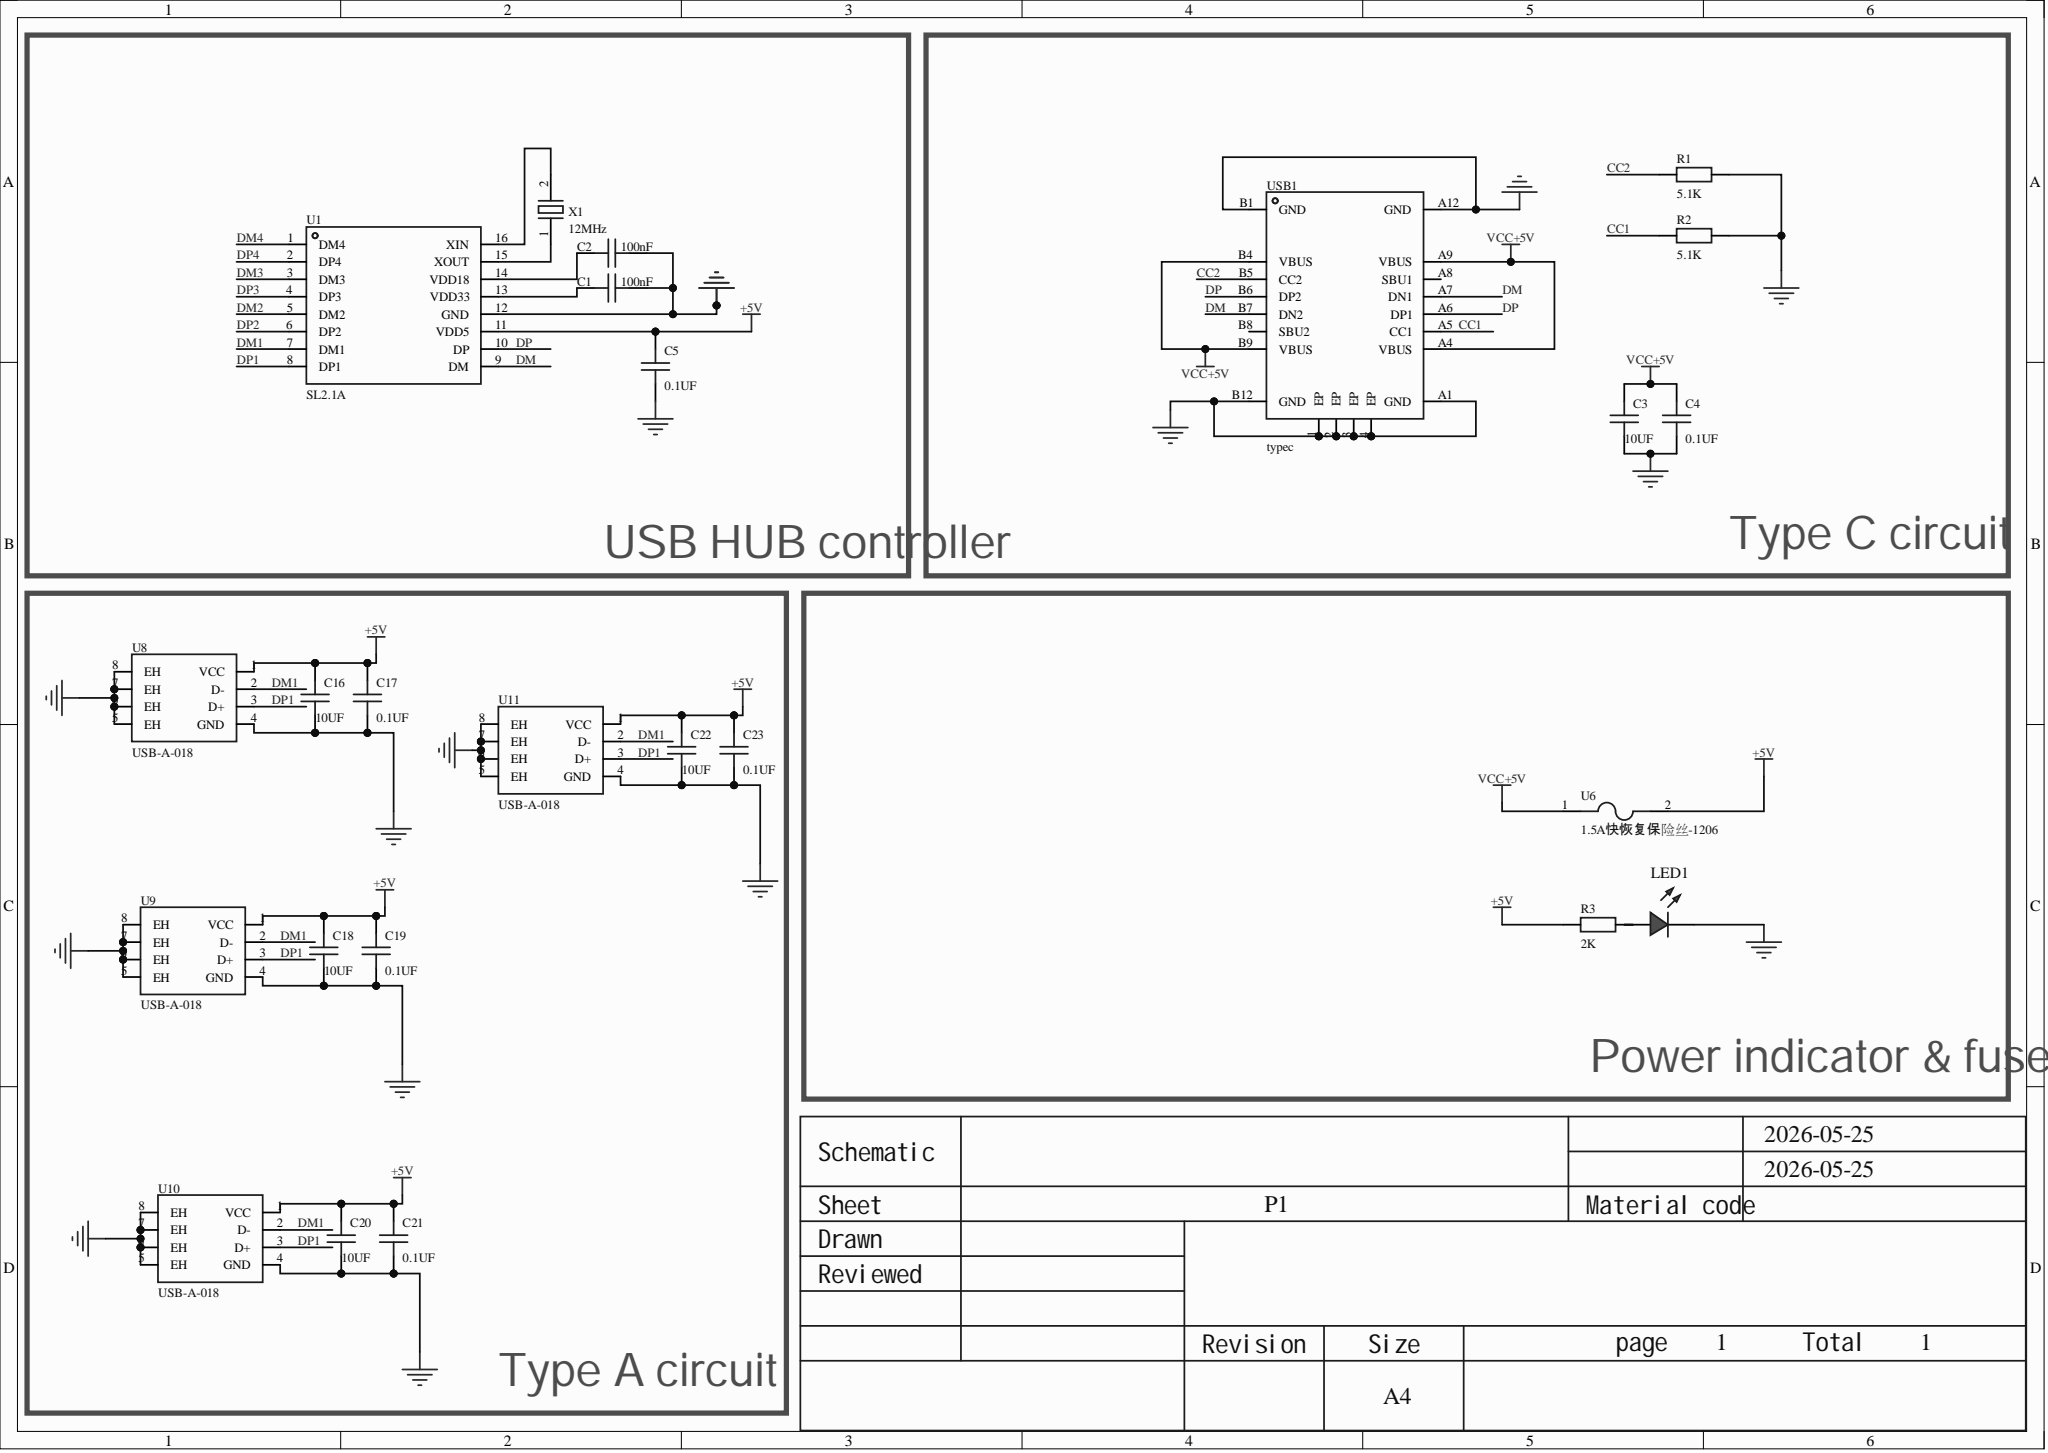Circuit board | Altium Designer | 25 parts | 14 nets
Bill of materials:
Comment,Description,Designator,Footprint,LibRef,Quantity
"100nF","","C1, C2","C0805","CAP_0805","2"
"10UF","","C3, C16, C18, C20, C22","C0805","CAP_0805","5"
"0.1UF","","C4, C5, C17, C19, C21, C23","C0805","CAP_0805","6"
"","","LED1","LED_0805","LED_0805-R","1"
"5.1K","","R1, R2","R0805","Res_0805","2"
"2K","","R3","R0805","Res_0805","1"
"SL2.1A","Application function: hub; interface protocol: -;","U1","SOP-16_L10.0-W3.9-P1.27-LS6.0-BL","SL2.1A","1"
"1.5A快恢复保险丝-1206","","U6","F1206","1.5A快恢复保险丝-1206","1"
"USB-A-018","","U8, U9, U10, U11","usb-smd_usb-a-018","USB-A-018","4"
"typec","","USB1","USB-C-SMD_KH-TYPE-C-16P","typec","1"
"12MHz","Crystal type: SMD crystal; frequency: 12MHz; frequency tolerance at room temperature: ±10ppm; external load capacitance: 20pF;","X1","CRYSTAL-SMD_L11.1-W4.8-LS12.3","9AT12000201060C3","1"
Netlist (Protel format):
[
C1
C0805
100nF



]
[
C2
C0805
100nF



]
[
C3
C0805
10UF



]
[
C4
C0805
0.1UF



]
[
C5
C0805
0.1UF



]
[
C16
C0805
10UF



]
[
C17
C0805
0.1UF



]
[
C18
C0805
10UF



]
[
C19
C0805
0.1UF



]
[
C20
C0805
10UF



]
[
C21
C0805
0.1UF



]
[
C22
C0805
10UF



]
[
C23
C0805
0.1UF



]
[
LED1
LED_0805




]
[
R1
R0805
5.1K



]
[
R2
R0805
5.1K



]
[
R3
R0805
2K



]
[
U1
SOP-16_L10.0-W3.9-P1.27-LS6.0-BL
SL2.1A



]
[
U6
F1206
1.5A快恢复保险丝-1206



]
[
U8
usb-smd_usb-a-018
USB-A-018



]
[
U9
usb-smd_usb-a-018
USB-A-018



]
[
U10
usb-smd_usb-a-018
USB-A-018



]
[
U11
usb-smd_usb-a-018
USB-A-018



]
[
USB1
USB-C-SMD_KH-TYPE-C-16P
typec



]
[
X1
CRYSTAL-SMD_L11.1-W4.8-LS12.3
12MHz



]
(
VCC+5V
C3-2
C4-2
U6-1
USB1-A4
USB1-A9
USB1-B4
USB1-B9
)
(
NetU1_16
U1-16
X1-2
)
(
NetU1_15
U1-15
X1-1
)
(
NetLED1_2
LED1-2
R3-1
)
(
NetC2_1
C2-1
U1-14
)
(
NetC1_1
C1-1
U1-13
)
(
GND
C1-2
C2-2
C3-1
C4-1
C5-1
C16-1
C17-1
C18-1
C19-1
C20-1
C21-1
C22-1
C23-1
LED1-1
R1-2
R2-2
U1-12
U8-4
U8-5
U8-6
U8-7
U8-8
U9-4
U9-5
U9-6
U9-7
U9-8
U10-4
U10-5
U10-6
U10-7
U10-8
U11-4
U11-5
U11-6
U11-7
U11-8
USB1-1
USB1-2
USB1-3
USB1-4
USB1-A1
USB1-A12
USB1-B1
USB1-B12
)
(
DP1
U1-8
U8-3
U9-3
U10-3
U11-3
)
(
DP
U1-10
USB1-A6
USB1-B6
)
(
DM1
U1-7
U8-2
U9-2
U10-2
U11-2
)
(
DM
U1-9
USB1-A7
USB1-B7
)
(
CC2
R1-1
USB1-B5
)
(
CC1
R2-1
USB1-A5
)
(
+5V
C5-2
C16-2
C17-2
C18-2
C19-2
C20-2
C21-2
C22-2
C23-2
R3-2
U1-11
U6-2
U8-1
U9-1
U10-1
U11-1
)